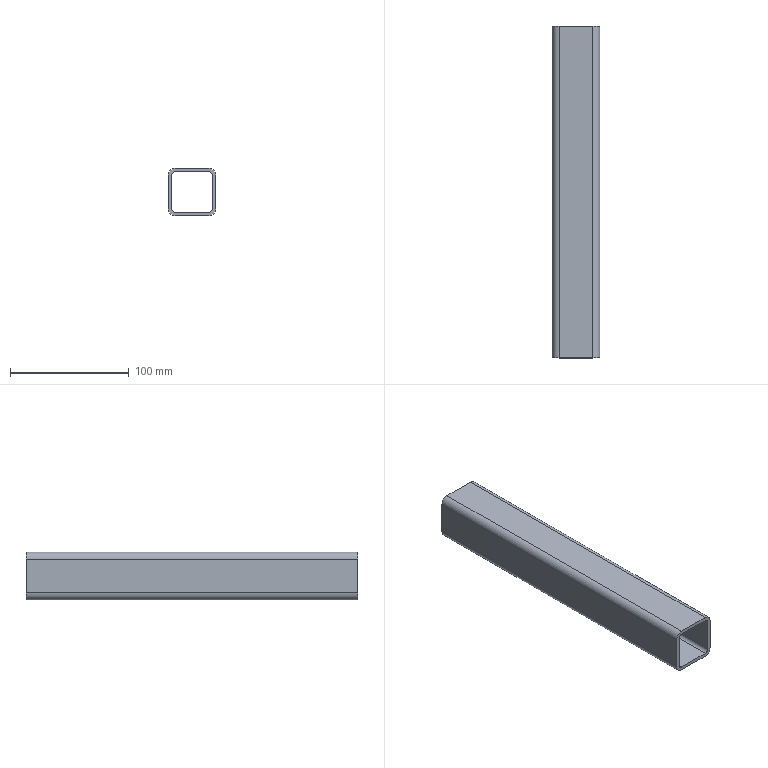Part | STEP file | SN10_002_008-05_TUBO_QUADRADO | 1 solid | 18 faces | box 40 x 280 x 40 mm | volume 117830 mm3 | plane 10 | cylinder 8 | commonest cylinder face diameters 6 x4 12 x4
STEP:
#1=CARTESIAN_POINT('',(0.,0.,0.));
#2=DIRECTION('',(0.,0.,1.));
#3=DIRECTION('',(1.,0.,0.));
#4=AXIS2_PLACEMENT_3D('',#1,#2,#3);
#5=CARTESIAN_POINT('',(14.,-140.,20.));
#6=VERTEX_POINT('',#5);
#7=CARTESIAN_POINT('',(14.,140.,20.));
#8=VERTEX_POINT('',#7);
#9=CARTESIAN_POINT('',(14.,-140.,20.));
#10=DIRECTION('',(0.,1.,0.));
#11=VECTOR('',#10,1.);
#12=LINE('',#9,#11);
#13=CARTESIAN_POINT('',(14.,0.,14.));
#14=DIRECTION('',(0.,1.,0.));
#15=DIRECTION('',(0.,0.,1.));
#16=AXIS2_PLACEMENT_3D('',#13,#14,#15);
#17=CYLINDRICAL_SURFACE('',#16,6.);
#18=CARTESIAN_POINT('',(0.,-140.));
#19=DIRECTION('',(0.,1.));
#20=VECTOR('',#19,1.);
#21=LINE('',#18,#20);
#22=(GEOMETRIC_REPRESENTATION_CONTEXT(2)PARAMETRIC_REPRESENTATION_CONTEXT()REPRESENTATION_CONTEXT('',''));
#23=DEFINITIONAL_REPRESENTATION('',(#21),#22);
#24=PCURVE('',#17,#23);
#25=CARTESIAN_POINT('',(14.,0.,20.));
#26=DIRECTION('',(0.,0.,-1.));
#27=DIRECTION('',(-1.,0.,0.));
#28=AXIS2_PLACEMENT_3D('',#25,#26,#27);
#29=PLANE('',#28);
#30=CARTESIAN_POINT('',(0.,-140.));
#31=DIRECTION('',(0.,1.));
#32=VECTOR('',#31,1.);
#33=LINE('',#30,#32);
#34=(GEOMETRIC_REPRESENTATION_CONTEXT(2)PARAMETRIC_REPRESENTATION_CONTEXT()REPRESENTATION_CONTEXT('',''));
#35=DEFINITIONAL_REPRESENTATION('',(#33),#34);
#36=PCURVE('',#29,#35);
#37=SURFACE_CURVE('',#12,(#24,#36),.PCURVE_S1.);
#38=EDGE_CURVE('',#6,#8,#37,.T.);
#39=ORIENTED_EDGE('',*,*,#38,.F.);
#40=CARTESIAN_POINT('',(20.,-140.,14.));
#41=VERTEX_POINT('',#40);
#42=CARTESIAN_POINT('',(14.,-140.,14.));
#43=DIRECTION('',(0.,1.,0.));
#44=DIRECTION('',(1.,0.,0.));
#45=AXIS2_PLACEMENT_3D('',#42,#43,#44);
#46=CIRCLE('',#45,6.);
#47=CARTESIAN_POINT('',(-4.712,-140.));
#48=DIRECTION('',(1.,0.));
#49=VECTOR('',#48,1.);
#50=LINE('',#47,#49);
#51=(GEOMETRIC_REPRESENTATION_CONTEXT(2)PARAMETRIC_REPRESENTATION_CONTEXT()REPRESENTATION_CONTEXT('',''));
#52=DEFINITIONAL_REPRESENTATION('',(#50),#51);
#53=PCURVE('',#17,#52);
#54=CARTESIAN_POINT('',(0.,-140.,0.));
#55=DIRECTION('',(0.,1.,0.));
#56=DIRECTION('',(0.,0.,1.));
#57=AXIS2_PLACEMENT_3D('',#54,#55,#56);
#58=PLANE('',#57);
#59=CARTESIAN_POINT('',(14.,14.));
#60=DIRECTION('',(0.,1.));
#61=AXIS2_PLACEMENT_2D('',#59,#60);
#62=CIRCLE('',#61,6.);
#63=(GEOMETRIC_REPRESENTATION_CONTEXT(2)PARAMETRIC_REPRESENTATION_CONTEXT()REPRESENTATION_CONTEXT('',''));
#64=DEFINITIONAL_REPRESENTATION('',(#62),#63);
#65=PCURVE('',#58,#64);
#66=SURFACE_CURVE('',#46,(#53,#65),.PCURVE_S1.);
#67=EDGE_CURVE('',#6,#41,#66,.T.);
#68=ORIENTED_EDGE('',*,*,#67,.T.);
#69=CARTESIAN_POINT('',(20.,140.,14.));
#70=VERTEX_POINT('',#69);
#71=CARTESIAN_POINT('',(20.,-140.,14.));
#72=DIRECTION('',(0.,1.,0.));
#73=VECTOR('',#72,1.);
#74=LINE('',#71,#73);
#75=CARTESIAN_POINT('',(1.571,-140.));
#76=DIRECTION('',(0.,1.));
#77=VECTOR('',#76,1.);
#78=LINE('',#75,#77);
#79=(GEOMETRIC_REPRESENTATION_CONTEXT(2)PARAMETRIC_REPRESENTATION_CONTEXT()REPRESENTATION_CONTEXT('',''));
#80=DEFINITIONAL_REPRESENTATION('',(#78),#79);
#81=PCURVE('',#17,#80);
#82=CARTESIAN_POINT('',(20.,0.,-14.));
#83=DIRECTION('',(-1.,0.,0.));
#84=DIRECTION('',(0.,0.,1.));
#85=AXIS2_PLACEMENT_3D('',#82,#83,#84);
#86=PLANE('',#85);
#87=CARTESIAN_POINT('',(28.,-140.));
#88=DIRECTION('',(0.,1.));
#89=VECTOR('',#88,1.);
#90=LINE('',#87,#89);
#91=(GEOMETRIC_REPRESENTATION_CONTEXT(2)PARAMETRIC_REPRESENTATION_CONTEXT()REPRESENTATION_CONTEXT('',''));
#92=DEFINITIONAL_REPRESENTATION('',(#90),#91);
#93=PCURVE('',#86,#92);
#94=SURFACE_CURVE('',#74,(#81,#93),.PCURVE_S1.);
#95=EDGE_CURVE('',#41,#70,#94,.T.);
#96=ORIENTED_EDGE('',*,*,#95,.T.);
#97=CARTESIAN_POINT('',(14.,140.,14.));
#98=DIRECTION('',(0.,1.,0.));
#99=DIRECTION('',(1.,0.,0.));
#100=AXIS2_PLACEMENT_3D('',#97,#98,#99);
#101=CIRCLE('',#100,6.);
#102=CARTESIAN_POINT('',(-4.712,140.));
#103=DIRECTION('',(1.,0.));
#104=VECTOR('',#103,1.);
#105=LINE('',#102,#104);
#106=(GEOMETRIC_REPRESENTATION_CONTEXT(2)PARAMETRIC_REPRESENTATION_CONTEXT()REPRESENTATION_CONTEXT('',''));
#107=DEFINITIONAL_REPRESENTATION('',(#105),#106);
#108=PCURVE('',#17,#107);
#109=CARTESIAN_POINT('',(0.,140.,0.));
#110=DIRECTION('',(0.,1.,0.));
#111=DIRECTION('',(0.,0.,1.));
#112=AXIS2_PLACEMENT_3D('',#109,#110,#111);
#113=PLANE('',#112);
#114=CARTESIAN_POINT('',(14.,14.));
#115=DIRECTION('',(0.,1.));
#116=AXIS2_PLACEMENT_2D('',#114,#115);
#117=CIRCLE('',#116,6.);
#118=(GEOMETRIC_REPRESENTATION_CONTEXT(2)PARAMETRIC_REPRESENTATION_CONTEXT()REPRESENTATION_CONTEXT('',''));
#119=DEFINITIONAL_REPRESENTATION('',(#117),#118);
#120=PCURVE('',#113,#119);
#121=SURFACE_CURVE('',#101,(#108,#120),.PCURVE_S1.);
#122=EDGE_CURVE('',#8,#70,#121,.T.);
#123=ORIENTED_EDGE('',*,*,#122,.F.);
#124=EDGE_LOOP('',(#39,#68,#96,#123));
#125=FACE_BOUND('',#124,.T.);
#126=ADVANCED_FACE('',(#125),#17,.T.);
#127=ORIENTED_EDGE('',*,*,#95,.F.);
#128=CARTESIAN_POINT('',(20.,-140.,-14.));
#129=VERTEX_POINT('',#128);
#130=CARTESIAN_POINT('',(20.,-140.,-14.));
#131=DIRECTION('',(0.,0.,1.));
#132=VECTOR('',#131,1.);
#133=LINE('',#130,#132);
#134=CARTESIAN_POINT('',(0.,-140.));
#135=DIRECTION('',(1.,0.));
#136=VECTOR('',#135,1.);
#137=LINE('',#134,#136);
#138=(GEOMETRIC_REPRESENTATION_CONTEXT(2)PARAMETRIC_REPRESENTATION_CONTEXT()REPRESENTATION_CONTEXT('',''));
#139=DEFINITIONAL_REPRESENTATION('',(#137),#138);
#140=PCURVE('',#86,#139);
#141=CARTESIAN_POINT('',(-14.,20.));
#142=DIRECTION('',(1.,0.));
#143=VECTOR('',#142,1.);
#144=LINE('',#141,#143);
#145=(GEOMETRIC_REPRESENTATION_CONTEXT(2)PARAMETRIC_REPRESENTATION_CONTEXT()REPRESENTATION_CONTEXT('',''));
#146=DEFINITIONAL_REPRESENTATION('',(#144),#145);
#147=PCURVE('',#58,#146);
#148=SURFACE_CURVE('',#133,(#140,#147),.PCURVE_S1.);
#149=EDGE_CURVE('',#129,#41,#148,.T.);
#150=ORIENTED_EDGE('',*,*,#149,.F.);
#151=CARTESIAN_POINT('',(20.,140.,-14.));
#152=VERTEX_POINT('',#151);
#153=CARTESIAN_POINT('',(20.,-140.,-14.));
#154=DIRECTION('',(0.,1.,0.));
#155=VECTOR('',#154,1.);
#156=LINE('',#153,#155);
#157=CARTESIAN_POINT('',(0.,-140.));
#158=DIRECTION('',(0.,1.));
#159=VECTOR('',#158,1.);
#160=LINE('',#157,#159);
#161=(GEOMETRIC_REPRESENTATION_CONTEXT(2)PARAMETRIC_REPRESENTATION_CONTEXT()REPRESENTATION_CONTEXT('',''));
#162=DEFINITIONAL_REPRESENTATION('',(#160),#161);
#163=PCURVE('',#86,#162);
#164=CARTESIAN_POINT('',(14.,0.,-14.));
#165=DIRECTION('',(0.,1.,0.));
#166=DIRECTION('',(1.,0.,0.));
#167=AXIS2_PLACEMENT_3D('',#164,#165,#166);
#168=CYLINDRICAL_SURFACE('',#167,6.);
#169=CARTESIAN_POINT('',(0.,-140.));
#170=DIRECTION('',(0.,1.));
#171=VECTOR('',#170,1.);
#172=LINE('',#169,#171);
#173=(GEOMETRIC_REPRESENTATION_CONTEXT(2)PARAMETRIC_REPRESENTATION_CONTEXT()REPRESENTATION_CONTEXT('',''));
#174=DEFINITIONAL_REPRESENTATION('',(#172),#173);
#175=PCURVE('',#168,#174);
#176=SURFACE_CURVE('',#156,(#163,#175),.PCURVE_S1.);
#177=EDGE_CURVE('',#129,#152,#176,.T.);
#178=ORIENTED_EDGE('',*,*,#177,.T.);
#179=CARTESIAN_POINT('',(20.,140.,-14.));
#180=DIRECTION('',(0.,0.,1.));
#181=VECTOR('',#180,1.);
#182=LINE('',#179,#181);
#183=CARTESIAN_POINT('',(0.,140.));
#184=DIRECTION('',(1.,0.));
#185=VECTOR('',#184,1.);
#186=LINE('',#183,#185);
#187=(GEOMETRIC_REPRESENTATION_CONTEXT(2)PARAMETRIC_REPRESENTATION_CONTEXT()REPRESENTATION_CONTEXT('',''));
#188=DEFINITIONAL_REPRESENTATION('',(#186),#187);
#189=PCURVE('',#86,#188);
#190=CARTESIAN_POINT('',(-14.,20.));
#191=DIRECTION('',(1.,0.));
#192=VECTOR('',#191,1.);
#193=LINE('',#190,#192);
#194=(GEOMETRIC_REPRESENTATION_CONTEXT(2)PARAMETRIC_REPRESENTATION_CONTEXT()REPRESENTATION_CONTEXT('',''));
#195=DEFINITIONAL_REPRESENTATION('',(#193),#194);
#196=PCURVE('',#113,#195);
#197=SURFACE_CURVE('',#182,(#189,#196),.PCURVE_S1.);
#198=EDGE_CURVE('',#152,#70,#197,.T.);
#199=ORIENTED_EDGE('',*,*,#198,.T.);
#200=EDGE_LOOP('',(#127,#150,#178,#199));
#201=FACE_BOUND('',#200,.T.);
#202=ADVANCED_FACE('',(#201),#86,.F.);
#203=ORIENTED_EDGE('',*,*,#177,.F.);
#204=CARTESIAN_POINT('',(14.,-140.,-20.));
#205=VERTEX_POINT('',#204);
#206=CARTESIAN_POINT('',(14.,-140.,-14.));
#207=DIRECTION('',(0.,1.,0.));
#208=DIRECTION('',(1.,0.,0.));
#209=AXIS2_PLACEMENT_3D('',#206,#207,#208);
#210=CIRCLE('',#209,6.);
#211=CARTESIAN_POINT('',(0.,-140.));
#212=DIRECTION('',(1.,0.));
#213=VECTOR('',#212,1.);
#214=LINE('',#211,#213);
#215=(GEOMETRIC_REPRESENTATION_CONTEXT(2)PARAMETRIC_REPRESENTATION_CONTEXT()REPRESENTATION_CONTEXT('',''));
#216=DEFINITIONAL_REPRESENTATION('',(#214),#215);
#217=PCURVE('',#168,#216);
#218=CARTESIAN_POINT('',(-14.,14.));
#219=DIRECTION('',(0.,1.));
#220=AXIS2_PLACEMENT_2D('',#218,#219);
#221=CIRCLE('',#220,6.);
#222=(GEOMETRIC_REPRESENTATION_CONTEXT(2)PARAMETRIC_REPRESENTATION_CONTEXT()REPRESENTATION_CONTEXT('',''));
#223=DEFINITIONAL_REPRESENTATION('',(#221),#222);
#224=PCURVE('',#58,#223);
#225=SURFACE_CURVE('',#210,(#217,#224),.PCURVE_S1.);
#226=EDGE_CURVE('',#129,#205,#225,.T.);
#227=ORIENTED_EDGE('',*,*,#226,.T.);
#228=CARTESIAN_POINT('',(14.,140.,-20.));
#229=VERTEX_POINT('',#228);
#230=CARTESIAN_POINT('',(14.,-140.,-20.));
#231=DIRECTION('',(0.,1.,0.));
#232=VECTOR('',#231,1.);
#233=LINE('',#230,#232);
#234=CARTESIAN_POINT('',(1.571,-140.));
#235=DIRECTION('',(0.,1.));
#236=VECTOR('',#235,1.);
#237=LINE('',#234,#236);
#238=(GEOMETRIC_REPRESENTATION_CONTEXT(2)PARAMETRIC_REPRESENTATION_CONTEXT()REPRESENTATION_CONTEXT('',''));
#239=DEFINITIONAL_REPRESENTATION('',(#237),#238);
#240=PCURVE('',#168,#239);
#241=CARTESIAN_POINT('',(-14.,0.,-20.));
#242=DIRECTION('',(0.,0.,1.));
#243=DIRECTION('',(1.,0.,0.));
#244=AXIS2_PLACEMENT_3D('',#241,#242,#243);
#245=PLANE('',#244);
#246=CARTESIAN_POINT('',(28.,-140.));
#247=DIRECTION('',(0.,1.));
#248=VECTOR('',#247,1.);
#249=LINE('',#246,#248);
#250=(GEOMETRIC_REPRESENTATION_CONTEXT(2)PARAMETRIC_REPRESENTATION_CONTEXT()REPRESENTATION_CONTEXT('',''));
#251=DEFINITIONAL_REPRESENTATION('',(#249),#250);
#252=PCURVE('',#245,#251);
#253=SURFACE_CURVE('',#233,(#240,#252),.PCURVE_S1.);
#254=EDGE_CURVE('',#205,#229,#253,.T.);
#255=ORIENTED_EDGE('',*,*,#254,.T.);
#256=CARTESIAN_POINT('',(14.,140.,-14.));
#257=DIRECTION('',(0.,1.,0.));
#258=DIRECTION('',(1.,0.,0.));
#259=AXIS2_PLACEMENT_3D('',#256,#257,#258);
#260=CIRCLE('',#259,6.);
#261=CARTESIAN_POINT('',(0.,140.));
#262=DIRECTION('',(1.,0.));
#263=VECTOR('',#262,1.);
#264=LINE('',#261,#263);
#265=(GEOMETRIC_REPRESENTATION_CONTEXT(2)PARAMETRIC_REPRESENTATION_CONTEXT()REPRESENTATION_CONTEXT('',''));
#266=DEFINITIONAL_REPRESENTATION('',(#264),#265);
#267=PCURVE('',#168,#266);
#268=CARTESIAN_POINT('',(-14.,14.));
#269=DIRECTION('',(0.,1.));
#270=AXIS2_PLACEMENT_2D('',#268,#269);
#271=CIRCLE('',#270,6.);
#272=(GEOMETRIC_REPRESENTATION_CONTEXT(2)PARAMETRIC_REPRESENTATION_CONTEXT()REPRESENTATION_CONTEXT('',''));
#273=DEFINITIONAL_REPRESENTATION('',(#271),#272);
#274=PCURVE('',#113,#273);
#275=SURFACE_CURVE('',#260,(#267,#274),.PCURVE_S1.);
#276=EDGE_CURVE('',#152,#229,#275,.T.);
#277=ORIENTED_EDGE('',*,*,#276,.F.);
#278=EDGE_LOOP('',(#203,#227,#255,#277));
#279=FACE_BOUND('',#278,.T.);
#280=ADVANCED_FACE('',(#279),#168,.T.);
#281=ORIENTED_EDGE('',*,*,#254,.F.);
#282=CARTESIAN_POINT('',(-14.,-140.,-20.));
#283=VERTEX_POINT('',#282);
#284=CARTESIAN_POINT('',(-14.,-140.,-20.));
#285=DIRECTION('',(1.,0.,0.));
#286=VECTOR('',#285,1.);
#287=LINE('',#284,#286);
#288=CARTESIAN_POINT('',(0.,-140.));
#289=DIRECTION('',(1.,0.));
#290=VECTOR('',#289,1.);
#291=LINE('',#288,#290);
#292=(GEOMETRIC_REPRESENTATION_CONTEXT(2)PARAMETRIC_REPRESENTATION_CONTEXT()REPRESENTATION_CONTEXT('',''));
#293=DEFINITIONAL_REPRESENTATION('',(#291),#292);
#294=PCURVE('',#245,#293);
#295=CARTESIAN_POINT('',(-20.,-14.));
#296=DIRECTION('',(0.,1.));
#297=VECTOR('',#296,1.);
#298=LINE('',#295,#297);
#299=(GEOMETRIC_REPRESENTATION_CONTEXT(2)PARAMETRIC_REPRESENTATION_CONTEXT()REPRESENTATION_CONTEXT('',''));
#300=DEFINITIONAL_REPRESENTATION('',(#298),#299);
#301=PCURVE('',#58,#300);
#302=SURFACE_CURVE('',#287,(#294,#301),.PCURVE_S1.);
#303=EDGE_CURVE('',#283,#205,#302,.T.);
#304=ORIENTED_EDGE('',*,*,#303,.F.);
#305=CARTESIAN_POINT('',(-14.,140.,-20.));
#306=VERTEX_POINT('',#305);
#307=CARTESIAN_POINT('',(-14.,-140.,-20.));
#308=DIRECTION('',(0.,1.,0.));
#309=VECTOR('',#308,1.);
#310=LINE('',#307,#309);
#311=CARTESIAN_POINT('',(0.,-140.));
#312=DIRECTION('',(0.,1.));
#313=VECTOR('',#312,1.);
#314=LINE('',#311,#313);
#315=(GEOMETRIC_REPRESENTATION_CONTEXT(2)PARAMETRIC_REPRESENTATION_CONTEXT()REPRESENTATION_CONTEXT('',''));
#316=DEFINITIONAL_REPRESENTATION('',(#314),#315);
#317=PCURVE('',#245,#316);
#318=CARTESIAN_POINT('',(-14.,0.,-14.));
#319=DIRECTION('',(0.,1.,0.));
#320=DIRECTION('',(0.,0.,-1.));
#321=AXIS2_PLACEMENT_3D('',#318,#319,#320);
#322=CYLINDRICAL_SURFACE('',#321,6.);
#323=CARTESIAN_POINT('',(0.,-140.));
#324=DIRECTION('',(0.,1.));
#325=VECTOR('',#324,1.);
#326=LINE('',#323,#325);
#327=(GEOMETRIC_REPRESENTATION_CONTEXT(2)PARAMETRIC_REPRESENTATION_CONTEXT()REPRESENTATION_CONTEXT('',''));
#328=DEFINITIONAL_REPRESENTATION('',(#326),#327);
#329=PCURVE('',#322,#328);
#330=SURFACE_CURVE('',#310,(#317,#329),.PCURVE_S1.);
#331=EDGE_CURVE('',#283,#306,#330,.T.);
#332=ORIENTED_EDGE('',*,*,#331,.T.);
#333=CARTESIAN_POINT('',(-14.,140.,-20.));
#334=DIRECTION('',(1.,0.,0.));
#335=VECTOR('',#334,1.);
#336=LINE('',#333,#335);
#337=CARTESIAN_POINT('',(0.,140.));
#338=DIRECTION('',(1.,0.));
#339=VECTOR('',#338,1.);
#340=LINE('',#337,#339);
#341=(GEOMETRIC_REPRESENTATION_CONTEXT(2)PARAMETRIC_REPRESENTATION_CONTEXT()REPRESENTATION_CONTEXT('',''));
#342=DEFINITIONAL_REPRESENTATION('',(#340),#341);
#343=PCURVE('',#245,#342);
#344=CARTESIAN_POINT('',(-20.,-14.));
#345=DIRECTION('',(0.,1.));
#346=VECTOR('',#345,1.);
#347=LINE('',#344,#346);
#348=(GEOMETRIC_REPRESENTATION_CONTEXT(2)PARAMETRIC_REPRESENTATION_CONTEXT()REPRESENTATION_CONTEXT('',''));
#349=DEFINITIONAL_REPRESENTATION('',(#347),#348);
#350=PCURVE('',#113,#349);
#351=SURFACE_CURVE('',#336,(#343,#350),.PCURVE_S1.);
#352=EDGE_CURVE('',#306,#229,#351,.T.);
#353=ORIENTED_EDGE('',*,*,#352,.T.);
#354=EDGE_LOOP('',(#281,#304,#332,#353));
#355=FACE_BOUND('',#354,.T.);
#356=ADVANCED_FACE('',(#355),#245,.F.);
#357=ORIENTED_EDGE('',*,*,#331,.F.);
#358=CARTESIAN_POINT('',(-20.,-140.,-14.));
#359=VERTEX_POINT('',#358);
#360=CARTESIAN_POINT('',(-14.,-140.,-14.));
#361=DIRECTION('',(0.,1.,0.));
#362=DIRECTION('',(1.,0.,0.));
#363=AXIS2_PLACEMENT_3D('',#360,#361,#362);
#364=CIRCLE('',#363,6.);
#365=CARTESIAN_POINT('',(-1.571,-140.));
#366=DIRECTION('',(1.,0.));
#367=VECTOR('',#366,1.);
#368=LINE('',#365,#367);
#369=(GEOMETRIC_REPRESENTATION_CONTEXT(2)PARAMETRIC_REPRESENTATION_CONTEXT()REPRESENTATION_CONTEXT('',''));
#370=DEFINITIONAL_REPRESENTATION('',(#368),#369);
#371=PCURVE('',#322,#370);
#372=CARTESIAN_POINT('',(-14.,-14.));
#373=DIRECTION('',(0.,1.));
#374=AXIS2_PLACEMENT_2D('',#372,#373);
#375=CIRCLE('',#374,6.);
#376=(GEOMETRIC_REPRESENTATION_CONTEXT(2)PARAMETRIC_REPRESENTATION_CONTEXT()REPRESENTATION_CONTEXT('',''));
#377=DEFINITIONAL_REPRESENTATION('',(#375),#376);
#378=PCURVE('',#58,#377);
#379=SURFACE_CURVE('',#364,(#371,#378),.PCURVE_S1.);
#380=EDGE_CURVE('',#283,#359,#379,.T.);
#381=ORIENTED_EDGE('',*,*,#380,.T.);
#382=CARTESIAN_POINT('',(-20.,140.,-14.));
#383=VERTEX_POINT('',#382);
#384=CARTESIAN_POINT('',(-20.,-140.,-14.));
#385=DIRECTION('',(0.,1.,0.));
#386=VECTOR('',#385,1.);
#387=LINE('',#384,#386);
#388=CARTESIAN_POINT('',(1.571,-140.));
#389=DIRECTION('',(0.,1.));
#390=VECTOR('',#389,1.);
#391=LINE('',#388,#390);
#392=(GEOMETRIC_REPRESENTATION_CONTEXT(2)PARAMETRIC_REPRESENTATION_CONTEXT()REPRESENTATION_CONTEXT('',''));
#393=DEFINITIONAL_REPRESENTATION('',(#391),#392);
#394=PCURVE('',#322,#393);
#395=CARTESIAN_POINT('',(-20.,0.,14.));
#396=DIRECTION('',(1.,0.,0.));
#397=DIRECTION('',(0.,0.,-1.));
#398=AXIS2_PLACEMENT_3D('',#395,#396,#397);
#399=PLANE('',#398);
#400=CARTESIAN_POINT('',(28.,-140.));
#401=DIRECTION('',(0.,1.));
#402=VECTOR('',#401,1.);
#403=LINE('',#400,#402);
#404=(GEOMETRIC_REPRESENTATION_CONTEXT(2)PARAMETRIC_REPRESENTATION_CONTEXT()REPRESENTATION_CONTEXT('',''));
#405=DEFINITIONAL_REPRESENTATION('',(#403),#404);
#406=PCURVE('',#399,#405);
#407=SURFACE_CURVE('',#387,(#394,#406),.PCURVE_S1.);
#408=EDGE_CURVE('',#359,#383,#407,.T.);
#409=ORIENTED_EDGE('',*,*,#408,.T.);
#410=CARTESIAN_POINT('',(-14.,140.,-14.));
#411=DIRECTION('',(0.,1.,0.));
#412=DIRECTION('',(1.,0.,0.));
#413=AXIS2_PLACEMENT_3D('',#410,#411,#412);
#414=CIRCLE('',#413,6.);
#415=CARTESIAN_POINT('',(-1.571,140.));
#416=DIRECTION('',(1.,0.));
#417=VECTOR('',#416,1.);
#418=LINE('',#415,#417);
#419=(GEOMETRIC_REPRESENTATION_CONTEXT(2)PARAMETRIC_REPRESENTATION_CONTEXT()REPRESENTATION_CONTEXT('',''));
#420=DEFINITIONAL_REPRESENTATION('',(#418),#419);
#421=PCURVE('',#322,#420);
#422=CARTESIAN_POINT('',(-14.,-14.));
#423=DIRECTION('',(0.,1.));
#424=AXIS2_PLACEMENT_2D('',#422,#423);
#425=CIRCLE('',#424,6.);
#426=(GEOMETRIC_REPRESENTATION_CONTEXT(2)PARAMETRIC_REPRESENTATION_CONTEXT()REPRESENTATION_CONTEXT('',''));
#427=DEFINITIONAL_REPRESENTATION('',(#425),#426);
#428=PCURVE('',#113,#427);
#429=SURFACE_CURVE('',#414,(#421,#428),.PCURVE_S1.);
#430=EDGE_CURVE('',#306,#383,#429,.T.);
#431=ORIENTED_EDGE('',*,*,#430,.F.);
#432=EDGE_LOOP('',(#357,#381,#409,#431));
#433=FACE_BOUND('',#432,.T.);
#434=ADVANCED_FACE('',(#433),#322,.T.);
#435=ORIENTED_EDGE('',*,*,#408,.F.);
#436=CARTESIAN_POINT('',(-20.,-140.,14.));
#437=VERTEX_POINT('',#436);
#438=CARTESIAN_POINT('',(-20.,-140.,14.));
#439=DIRECTION('',(0.,0.,-1.));
#440=VECTOR('',#439,1.);
#441=LINE('',#438,#440);
#442=CARTESIAN_POINT('',(0.,-140.));
#443=DIRECTION('',(1.,0.));
#444=VECTOR('',#443,1.);
#445=LINE('',#442,#444);
#446=(GEOMETRIC_REPRESENTATION_CONTEXT(2)PARAMETRIC_REPRESENTATION_CONTEXT()REPRESENTATION_CONTEXT('',''));
#447=DEFINITIONAL_REPRESENTATION('',(#445),#446);
#448=PCURVE('',#399,#447);
#449=CARTESIAN_POINT('',(14.,-20.));
#450=DIRECTION('',(-1.,0.));
#451=VECTOR('',#450,1.);
#452=LINE('',#449,#451);
#453=(GEOMETRIC_REPRESENTATION_CONTEXT(2)PARAMETRIC_REPRESENTATION_CONTEXT()REPRESENTATION_CONTEXT('',''));
#454=DEFINITIONAL_REPRESENTATION('',(#452),#453);
#455=PCURVE('',#58,#454);
#456=SURFACE_CURVE('',#441,(#448,#455),.PCURVE_S1.);
#457=EDGE_CURVE('',#437,#359,#456,.T.);
#458=ORIENTED_EDGE('',*,*,#457,.F.);
#459=CARTESIAN_POINT('',(-20.,140.,14.));
#460=VERTEX_POINT('',#459);
#461=CARTESIAN_POINT('',(-20.,-140.,14.));
#462=DIRECTION('',(0.,1.,0.));
#463=VECTOR('',#462,1.);
#464=LINE('',#461,#463);
#465=CARTESIAN_POINT('',(0.,-140.));
#466=DIRECTION('',(0.,1.));
#467=VECTOR('',#466,1.);
#468=LINE('',#465,#467);
#469=(GEOMETRIC_REPRESENTATION_CONTEXT(2)PARAMETRIC_REPRESENTATION_CONTEXT()REPRESENTATION_CONTEXT('',''));
#470=DEFINITIONAL_REPRESENTATION('',(#468),#469);
#471=PCURVE('',#399,#470);
#472=CARTESIAN_POINT('',(-14.,0.,14.));
#473=DIRECTION('',(0.,1.,0.));
#474=DIRECTION('',(-1.,0.,0.));
#475=AXIS2_PLACEMENT_3D('',#472,#473,#474);
#476=CYLINDRICAL_SURFACE('',#475,6.);
#477=CARTESIAN_POINT('',(0.,-140.));
#478=DIRECTION('',(0.,1.));
#479=VECTOR('',#478,1.);
#480=LINE('',#477,#479);
#481=(GEOMETRIC_REPRESENTATION_CONTEXT(2)PARAMETRIC_REPRESENTATION_CONTEXT()REPRESENTATION_CONTEXT('',''));
#482=DEFINITIONAL_REPRESENTATION('',(#480),#481);
#483=PCURVE('',#476,#482);
#484=SURFACE_CURVE('',#464,(#471,#483),.PCURVE_S1.);
#485=EDGE_CURVE('',#437,#460,#484,.T.);
#486=ORIENTED_EDGE('',*,*,#485,.T.);
#487=CARTESIAN_POINT('',(-20.,140.,14.));
#488=DIRECTION('',(0.,0.,-1.));
#489=VECTOR('',#488,1.);
#490=LINE('',#487,#489);
#491=CARTESIAN_POINT('',(0.,140.));
#492=DIRECTION('',(1.,0.));
#493=VECTOR('',#492,1.);
#494=LINE('',#491,#493);
#495=(GEOMETRIC_REPRESENTATION_CONTEXT(2)PARAMETRIC_REPRESENTATION_CONTEXT()REPRESENTATION_CONTEXT('',''));
#496=DEFINITIONAL_REPRESENTATION('',(#494),#495);
#497=PCURVE('',#399,#496);
#498=CARTESIAN_POINT('',(14.,-20.));
#499=DIRECTION('',(-1.,0.));
#500=VECTOR('',#499,1.);
#501=LINE('',#498,#500);
#502=(GEOMETRIC_REPRESENTATION_CONTEXT(2)PARAMETRIC_REPRESENTATION_CONTEXT()REPRESENTATION_CONTEXT('',''));
#503=DEFINITIONAL_REPRESENTATION('',(#501),#502);
#504=PCURVE('',#113,#503);
#505=SURFACE_CURVE('',#490,(#497,#504),.PCURVE_S1.);
#506=EDGE_CURVE('',#460,#383,#505,.T.);
#507=ORIENTED_EDGE('',*,*,#506,.T.);
#508=EDGE_LOOP('',(#435,#458,#486,#507));
#509=FACE_BOUND('',#508,.T.);
#510=ADVANCED_FACE('',(#509),#399,.F.);
#511=ORIENTED_EDGE('',*,*,#485,.F.);
#512=CARTESIAN_POINT('',(-14.,-140.,20.));
#513=VERTEX_POINT('',#512);
#514=CARTESIAN_POINT('',(-14.,-140.,14.));
#515=DIRECTION('',(0.,1.,0.));
#516=DIRECTION('',(1.,0.,0.));
#517=AXIS2_PLACEMENT_3D('',#514,#515,#516);
#518=CIRCLE('',#517,6.);
#519=CARTESIAN_POINT('',(-3.142,-140.));
#520=DIRECTION('',(1.,0.));
#521=VECTOR('',#520,1.);
#522=LINE('',#519,#521);
#523=(GEOMETRIC_REPRESENTATION_CONTEXT(2)PARAMETRIC_REPRESENTATION_CONTEXT()REPRESENTATION_CONTEXT('',''));
#524=DEFINITIONAL_REPRESENTATION('',(#522),#523);
#525=PCURVE('',#476,#524);
#526=CARTESIAN_POINT('',(14.,-14.));
#527=DIRECTION('',(0.,1.));
#528=AXIS2_PLACEMENT_2D('',#526,#527);
#529=CIRCLE('',#528,6.);
#530=(GEOMETRIC_REPRESENTATION_CONTEXT(2)PARAMETRIC_REPRESENTATION_CONTEXT()REPRESENTATION_CONTEXT('',''));
#531=DEFINITIONAL_REPRESENTATION('',(#529),#530);
#532=PCURVE('',#58,#531);
#533=SURFACE_CURVE('',#518,(#525,#532),.PCURVE_S1.);
#534=EDGE_CURVE('',#437,#513,#533,.T.);
#535=ORIENTED_EDGE('',*,*,#534,.T.);
#536=CARTESIAN_POINT('',(-14.,140.,20.));
#537=VERTEX_POINT('',#536);
#538=CARTESIAN_POINT('',(-14.,-140.,20.));
#539=DIRECTION('',(0.,1.,0.));
#540=VECTOR('',#539,1.);
#541=LINE('',#538,#540);
#542=CARTESIAN_POINT('',(1.571,-140.));
#543=DIRECTION('',(0.,1.));
#544=VECTOR('',#543,1.);
#545=LINE('',#542,#544);
#546=(GEOMETRIC_REPRESENTATION_CONTEXT(2)PARAMETRIC_REPRESENTATION_CONTEXT()REPRESENTATION_CONTEXT('',''));
#547=DEFINITIONAL_REPRESENTATION('',(#545),#546);
#548=PCURVE('',#476,#547);
#549=CARTESIAN_POINT('',(28.,-140.));
#550=DIRECTION('',(0.,1.));
#551=VECTOR('',#550,1.);
#552=LINE('',#549,#551);
#553=(GEOMETRIC_REPRESENTATION_CONTEXT(2)PARAMETRIC_REPRESENTATION_CONTEXT()REPRESENTATION_CONTEXT('',''));
#554=DEFINITIONAL_REPRESENTATION('',(#552),#553);
#555=PCURVE('',#29,#554);
#556=SURFACE_CURVE('',#541,(#548,#555),.PCURVE_S1.);
#557=EDGE_CURVE('',#513,#537,#556,.T.);
#558=ORIENTED_EDGE('',*,*,#557,.T.);
#559=CARTESIAN_POINT('',(-14.,140.,14.));
#560=DIRECTION('',(0.,1.,0.));
#561=DIRECTION('',(1.,0.,0.));
#562=AXIS2_PLACEMENT_3D('',#559,#560,#561);
#563=CIRCLE('',#562,6.);
#564=CARTESIAN_POINT('',(-3.142,140.));
#565=DIRECTION('',(1.,0.));
#566=VECTOR('',#565,1.);
#567=LINE('',#564,#566);
#568=(GEOMETRIC_REPRESENTATION_CONTEXT(2)PARAMETRIC_REPRESENTATION_CONTEXT()REPRESENTATION_CONTEXT('',''));
#569=DEFINITIONAL_REPRESENTATION('',(#567),#568);
#570=PCURVE('',#476,#569);
#571=CARTESIAN_POINT('',(14.,-14.));
#572=DIRECTION('',(0.,1.));
#573=AXIS2_PLACEMENT_2D('',#571,#572);
#574=CIRCLE('',#573,6.);
#575=(GEOMETRIC_REPRESENTATION_CONTEXT(2)PARAMETRIC_REPRESENTATION_CONTEXT()REPRESENTATION_CONTEXT('',''));
#576=DEFINITIONAL_REPRESENTATION('',(#574),#575);
#577=PCURVE('',#113,#576);
#578=SURFACE_CURVE('',#563,(#570,#577),.PCURVE_S1.);
#579=EDGE_CURVE('',#460,#537,#578,.T.);
#580=ORIENTED_EDGE('',*,*,#579,.F.);
#581=EDGE_LOOP('',(#511,#535,#558,#580));
#582=FACE_BOUND('',#581,.T.);
#583=ADVANCED_FACE('',(#582),#476,.T.);
#584=ORIENTED_EDGE('',*,*,#557,.F.);
#585=CARTESIAN_POINT('',(14.,-140.,20.));
#586=DIRECTION('',(-1.,0.,0.));
#587=VECTOR('',#586,1.);
#588=LINE('',#585,#587);
#589=CARTESIAN_POINT('',(0.,-140.));
#590=DIRECTION('',(1.,0.));
#591=VECTOR('',#590,1.);
#592=LINE('',#589,#591);
#593=(GEOMETRIC_REPRESENTATION_CONTEXT(2)PARAMETRIC_REPRESENTATION_CONTEXT()REPRESENTATION_CONTEXT('',''));
#594=DEFINITIONAL_REPRESENTATION('',(#592),#593);
#595=PCURVE('',#29,#594);
#596=CARTESIAN_POINT('',(20.,14.));
#597=DIRECTION('',(0.,-1.));
#598=VECTOR('',#597,1.);
#599=LINE('',#596,#598);
#600=(GEOMETRIC_REPRESENTATION_CONTEXT(2)PARAMETRIC_REPRESENTATION_CONTEXT()REPRESENTATION_CONTEXT('',''));
#601=DEFINITIONAL_REPRESENTATION('',(#599),#600);
#602=PCURVE('',#58,#601);
#603=SURFACE_CURVE('',#588,(#595,#602),.PCURVE_S1.);
#604=EDGE_CURVE('',#6,#513,#603,.T.);
#605=ORIENTED_EDGE('',*,*,#604,.F.);
#606=ORIENTED_EDGE('',*,*,#38,.T.);
#607=CARTESIAN_POINT('',(14.,140.,20.));
#608=DIRECTION('',(-1.,0.,0.));
#609=VECTOR('',#608,1.);
#610=LINE('',#607,#609);
#611=CARTESIAN_POINT('',(0.,140.));
#612=DIRECTION('',(1.,0.));
#613=VECTOR('',#612,1.);
#614=LINE('',#611,#613);
#615=(GEOMETRIC_REPRESENTATION_CONTEXT(2)PARAMETRIC_REPRESENTATION_CONTEXT()REPRESENTATION_CONTEXT('',''));
#616=DEFINITIONAL_REPRESENTATION('',(#614),#615);
#617=PCURVE('',#29,#616);
#618=CARTESIAN_POINT('',(20.,14.));
#619=DIRECTION('',(0.,-1.));
#620=VECTOR('',#619,1.);
#621=LINE('',#618,#620);
#622=(GEOMETRIC_REPRESENTATION_CONTEXT(2)PARAMETRIC_REPRESENTATION_CONTEXT()REPRESENTATION_CONTEXT('',''));
#623=DEFINITIONAL_REPRESENTATION('',(#621),#622);
#624=PCURVE('',#113,#623);
#625=SURFACE_CURVE('',#610,(#617,#624),.PCURVE_S1.);
#626=EDGE_CURVE('',#8,#537,#625,.T.);
#627=ORIENTED_EDGE('',*,*,#626,.T.);
#628=EDGE_LOOP('',(#584,#605,#606,#627));
#629=FACE_BOUND('',#628,.T.);
#630=ADVANCED_FACE('',(#629),#29,.F.);
#631=CARTESIAN_POINT('',(14.,140.,17.));
#632=VERTEX_POINT('',#631);
#633=CARTESIAN_POINT('',(-14.,140.,17.));
#634=VERTEX_POINT('',#633);
#635=CARTESIAN_POINT('',(14.,140.,17.));
#636=DIRECTION('',(-1.,0.,0.));
#637=VECTOR('',#636,1.);
#638=LINE('',#635,#637);
#639=CARTESIAN_POINT('',(14.,0.,17.));
#640=DIRECTION('',(0.,0.,-1.));
#641=DIRECTION('',(-1.,0.,0.));
#642=AXIS2_PLACEMENT_3D('',#639,#640,#641);
#643=PLANE('',#642);
#644=CARTESIAN_POINT('',(0.,140.));
#645=DIRECTION('',(1.,0.));
#646=VECTOR('',#645,1.);
#647=LINE('',#644,#646);
#648=(GEOMETRIC_REPRESENTATION_CONTEXT(2)PARAMETRIC_REPRESENTATION_CONTEXT()REPRESENTATION_CONTEXT('',''));
#649=DEFINITIONAL_REPRESENTATION('',(#647),#648);
#650=PCURVE('',#643,#649);
#651=CARTESIAN_POINT('',(17.,14.));
#652=DIRECTION('',(0.,-1.));
#653=VECTOR('',#652,1.);
#654=LINE('',#651,#653);
#655=(GEOMETRIC_REPRESENTATION_CONTEXT(2)PARAMETRIC_REPRESENTATION_CONTEXT()REPRESENTATION_CONTEXT('',''));
#656=DEFINITIONAL_REPRESENTATION('',(#654),#655);
#657=PCURVE('',#113,#656);
#658=SURFACE_CURVE('',#638,(#650,#657),.PCURVE_S1.);
#659=EDGE_CURVE('',#632,#634,#658,.T.);
#660=ORIENTED_EDGE('',*,*,#659,.F.);
#661=CARTESIAN_POINT('',(14.,-140.,17.));
#662=VERTEX_POINT('',#661);
#663=CARTESIAN_POINT('',(14.,-140.,17.));
#664=DIRECTION('',(0.,1.,0.));
#665=VECTOR('',#664,1.);
#666=LINE('',#663,#665);
#667=CARTESIAN_POINT('',(0.,-140.));
#668=DIRECTION('',(0.,1.));
#669=VECTOR('',#668,1.);
#670=LINE('',#667,#669);
#671=(GEOMETRIC_REPRESENTATION_CONTEXT(2)PARAMETRIC_REPRESENTATION_CONTEXT()REPRESENTATION_CONTEXT('',''));
#672=DEFINITIONAL_REPRESENTATION('',(#670),#671);
#673=PCURVE('',#643,#672);
#674=CARTESIAN_POINT('',(14.,0.,14.));
#675=DIRECTION('',(0.,1.,0.));
#676=DIRECTION('',(0.,0.,1.));
#677=AXIS2_PLACEMENT_3D('',#674,#675,#676);
#678=CYLINDRICAL_SURFACE('',#677,3.);
#679=CARTESIAN_POINT('',(0.,-140.));
#680=DIRECTION('',(0.,1.));
#681=VECTOR('',#680,1.);
#682=LINE('',#679,#681);
#683=(GEOMETRIC_REPRESENTATION_CONTEXT(2)PARAMETRIC_REPRESENTATION_CONTEXT()REPRESENTATION_CONTEXT('',''));
#684=DEFINITIONAL_REPRESENTATION('',(#682),#683);
#685=PCURVE('',#678,#684);
#686=SURFACE_CURVE('',#666,(#673,#685),.PCURVE_S1.);
#687=EDGE_CURVE('',#662,#632,#686,.T.);
#688=ORIENTED_EDGE('',*,*,#687,.F.);
#689=CARTESIAN_POINT('',(-14.,-140.,17.));
#690=VERTEX_POINT('',#689);
#691=CARTESIAN_POINT('',(14.,-140.,17.));
#692=DIRECTION('',(-1.,0.,0.));
#693=VECTOR('',#692,1.);
#694=LINE('',#691,#693);
#695=CARTESIAN_POINT('',(0.,-140.));
#696=DIRECTION('',(1.,0.));
#697=VECTOR('',#696,1.);
#698=LINE('',#695,#697);
#699=(GEOMETRIC_REPRESENTATION_CONTEXT(2)PARAMETRIC_REPRESENTATION_CONTEXT()REPRESENTATION_CONTEXT('',''));
#700=DEFINITIONAL_REPRESENTATION('',(#698),#699);
#701=PCURVE('',#643,#700);
#702=CARTESIAN_POINT('',(17.,14.));
#703=DIRECTION('',(0.,-1.));
#704=VECTOR('',#703,1.);
#705=LINE('',#702,#704);
#706=(GEOMETRIC_REPRESENTATION_CONTEXT(2)PARAMETRIC_REPRESENTATION_CONTEXT()REPRESENTATION_CONTEXT('',''));
#707=DEFINITIONAL_REPRESENTATION('',(#705),#706);
#708=PCURVE('',#58,#707);
#709=SURFACE_CURVE('',#694,(#701,#708),.PCURVE_S1.);
#710=EDGE_CURVE('',#662,#690,#709,.T.);
#711=ORIENTED_EDGE('',*,*,#710,.T.);
#712=CARTESIAN_POINT('',(-14.,-140.,17.));
#713=DIRECTION('',(0.,1.,0.));
#714=VECTOR('',#713,1.);
#715=LINE('',#712,#714);
#716=CARTESIAN_POINT('',(28.,-140.));
#717=DIRECTION('',(0.,1.));
#718=VECTOR('',#717,1.);
#719=LINE('',#716,#718);
#720=(GEOMETRIC_REPRESENTATION_CONTEXT(2)PARAMETRIC_REPRESENTATION_CONTEXT()REPRESENTATION_CONTEXT('',''));
#721=DEFINITIONAL_REPRESENTATION('',(#719),#720);
#722=PCURVE('',#643,#721);
#723=CARTESIAN_POINT('',(-14.,0.,14.));
#724=DIRECTION('',(0.,1.,0.));
#725=DIRECTION('',(-1.,0.,0.));
#726=AXIS2_PLACEMENT_3D('',#723,#724,#725);
#727=CYLINDRICAL_SURFACE('',#726,3.);
#728=CARTESIAN_POINT('',(1.571,-140.));
#729=DIRECTION('',(0.,1.));
#730=VECTOR('',#729,1.);
#731=LINE('',#728,#730);
#732=(GEOMETRIC_REPRESENTATION_CONTEXT(2)PARAMETRIC_REPRESENTATION_CONTEXT()REPRESENTATION_CONTEXT('',''));
#733=DEFINITIONAL_REPRESENTATION('',(#731),#732);
#734=PCURVE('',#727,#733);
#735=SURFACE_CURVE('',#715,(#722,#734),.PCURVE_S1.);
#736=EDGE_CURVE('',#690,#634,#735,.T.);
#737=ORIENTED_EDGE('',*,*,#736,.T.);
#738=EDGE_LOOP('',(#660,#688,#711,#737));
#739=FACE_BOUND('',#738,.T.);
#740=ADVANCED_FACE('',(#739),#643,.T.);
#741=CARTESIAN_POINT('',(-17.,-140.,14.));
#742=VERTEX_POINT('',#741);
#743=CARTESIAN_POINT('',(-17.,140.,14.));
#744=VERTEX_POINT('',#743);
#745=CARTESIAN_POINT('',(-17.,-140.,14.));
#746=DIRECTION('',(0.,1.,0.));
#747=VECTOR('',#746,1.);
#748=LINE('',#745,#747);
#749=CARTESIAN_POINT('',(0.,-140.));
#750=DIRECTION('',(0.,1.));
#751=VECTOR('',#750,1.);
#752=LINE('',#749,#751);
#753=(GEOMETRIC_REPRESENTATION_CONTEXT(2)PARAMETRIC_REPRESENTATION_CONTEXT()REPRESENTATION_CONTEXT('',''));
#754=DEFINITIONAL_REPRESENTATION('',(#752),#753);
#755=PCURVE('',#727,#754);
#756=CARTESIAN_POINT('',(-17.,0.,14.));
#757=DIRECTION('',(1.,0.,0.));
#758=DIRECTION('',(0.,0.,-1.));
#759=AXIS2_PLACEMENT_3D('',#756,#757,#758);
#760=PLANE('',#759);
#761=CARTESIAN_POINT('',(0.,-140.));
#762=DIRECTION('',(0.,1.));
#763=VECTOR('',#762,1.);
#764=LINE('',#761,#763);
#765=(GEOMETRIC_REPRESENTATION_CONTEXT(2)PARAMETRIC_REPRESENTATION_CONTEXT()REPRESENTATION_CONTEXT('',''));
#766=DEFINITIONAL_REPRESENTATION('',(#764),#765);
#767=PCURVE('',#760,#766);
#768=SURFACE_CURVE('',#748,(#755,#767),.PCURVE_S1.);
#769=EDGE_CURVE('',#742,#744,#768,.T.);
#770=ORIENTED_EDGE('',*,*,#769,.F.);
#771=CARTESIAN_POINT('',(-14.,-140.,14.));
#772=DIRECTION('',(0.,1.,0.));
#773=DIRECTION('',(1.,0.,0.));
#774=AXIS2_PLACEMENT_3D('',#771,#772,#773);
#775=CIRCLE('',#774,3.);
#776=CARTESIAN_POINT('',(-3.142,-140.));
#777=DIRECTION('',(1.,0.));
#778=VECTOR('',#777,1.);
#779=LINE('',#776,#778);
#780=(GEOMETRIC_REPRESENTATION_CONTEXT(2)PARAMETRIC_REPRESENTATION_CONTEXT()REPRESENTATION_CONTEXT('',''));
#781=DEFINITIONAL_REPRESENTATION('',(#779),#780);
#782=PCURVE('',#727,#781);
#783=CARTESIAN_POINT('',(14.,-14.));
#784=DIRECTION('',(0.,1.));
#785=AXIS2_PLACEMENT_2D('',#783,#784);
#786=CIRCLE('',#785,3.);
#787=(GEOMETRIC_REPRESENTATION_CONTEXT(2)PARAMETRIC_REPRESENTATION_CONTEXT()REPRESENTATION_CONTEXT('',''));
#788=DEFINITIONAL_REPRESENTATION('',(#786),#787);
#789=PCURVE('',#58,#788);
#790=SURFACE_CURVE('',#775,(#782,#789),.PCURVE_S1.);
#791=EDGE_CURVE('',#742,#690,#790,.T.);
#792=ORIENTED_EDGE('',*,*,#791,.T.);
#793=ORIENTED_EDGE('',*,*,#736,.T.);
#794=CARTESIAN_POINT('',(-14.,140.,14.));
#795=DIRECTION('',(0.,1.,0.));
#796=DIRECTION('',(1.,0.,0.));
#797=AXIS2_PLACEMENT_3D('',#794,#795,#796);
#798=CIRCLE('',#797,3.);
#799=CARTESIAN_POINT('',(-3.142,140.));
#800=DIRECTION('',(1.,0.));
#801=VECTOR('',#800,1.);
#802=LINE('',#799,#801);
#803=(GEOMETRIC_REPRESENTATION_CONTEXT(2)PARAMETRIC_REPRESENTATION_CONTEXT()REPRESENTATION_CONTEXT('',''));
#804=DEFINITIONAL_REPRESENTATION('',(#802),#803);
#805=PCURVE('',#727,#804);
#806=CARTESIAN_POINT('',(14.,-14.));
#807=DIRECTION('',(0.,1.));
#808=AXIS2_PLACEMENT_2D('',#806,#807);
#809=CIRCLE('',#808,3.);
#810=(GEOMETRIC_REPRESENTATION_CONTEXT(2)PARAMETRIC_REPRESENTATION_CONTEXT()REPRESENTATION_CONTEXT('',''));
#811=DEFINITIONAL_REPRESENTATION('',(#809),#810);
#812=PCURVE('',#113,#811);
#813=SURFACE_CURVE('',#798,(#805,#812),.PCURVE_S1.);
#814=EDGE_CURVE('',#744,#634,#813,.T.);
#815=ORIENTED_EDGE('',*,*,#814,.F.);
#816=EDGE_LOOP('',(#770,#792,#793,#815));
#817=FACE_BOUND('',#816,.F.);
#818=ADVANCED_FACE('',(#817),#727,.F.);
#819=CARTESIAN_POINT('',(-17.,140.,-14.));
#820=VERTEX_POINT('',#819);
#821=CARTESIAN_POINT('',(-17.,140.,14.));
#822=DIRECTION('',(0.,0.,-1.));
#823=VECTOR('',#822,1.);
#824=LINE('',#821,#823);
#825=CARTESIAN_POINT('',(0.,140.));
#826=DIRECTION('',(1.,0.));
#827=VECTOR('',#826,1.);
#828=LINE('',#825,#827);
#829=(GEOMETRIC_REPRESENTATION_CONTEXT(2)PARAMETRIC_REPRESENTATION_CONTEXT()REPRESENTATION_CONTEXT('',''));
#830=DEFINITIONAL_REPRESENTATION('',(#828),#829);
#831=PCURVE('',#760,#830);
#832=CARTESIAN_POINT('',(14.,-17.));
#833=DIRECTION('',(-1.,0.));
#834=VECTOR('',#833,1.);
#835=LINE('',#832,#834);
#836=(GEOMETRIC_REPRESENTATION_CONTEXT(2)PARAMETRIC_REPRESENTATION_CONTEXT()REPRESENTATION_CONTEXT('',''));
#837=DEFINITIONAL_REPRESENTATION('',(#835),#836);
#838=PCURVE('',#113,#837);
#839=SURFACE_CURVE('',#824,(#831,#838),.PCURVE_S1.);
#840=EDGE_CURVE('',#744,#820,#839,.T.);
#841=ORIENTED_EDGE('',*,*,#840,.F.);
#842=ORIENTED_EDGE('',*,*,#769,.F.);
#843=CARTESIAN_POINT('',(-17.,-140.,-14.));
#844=VERTEX_POINT('',#843);
#845=CARTESIAN_POINT('',(-17.,-140.,14.));
#846=DIRECTION('',(0.,0.,-1.));
#847=VECTOR('',#846,1.);
#848=LINE('',#845,#847);
#849=CARTESIAN_POINT('',(0.,-140.));
#850=DIRECTION('',(1.,0.));
#851=VECTOR('',#850,1.);
#852=LINE('',#849,#851);
#853=(GEOMETRIC_REPRESENTATION_CONTEXT(2)PARAMETRIC_REPRESENTATION_CONTEXT()REPRESENTATION_CONTEXT('',''));
#854=DEFINITIONAL_REPRESENTATION('',(#852),#853);
#855=PCURVE('',#760,#854);
#856=CARTESIAN_POINT('',(14.,-17.));
#857=DIRECTION('',(-1.,0.));
#858=VECTOR('',#857,1.);
#859=LINE('',#856,#858);
#860=(GEOMETRIC_REPRESENTATION_CONTEXT(2)PARAMETRIC_REPRESENTATION_CONTEXT()REPRESENTATION_CONTEXT('',''));
#861=DEFINITIONAL_REPRESENTATION('',(#859),#860);
#862=PCURVE('',#58,#861);
#863=SURFACE_CURVE('',#848,(#855,#862),.PCURVE_S1.);
#864=EDGE_CURVE('',#742,#844,#863,.T.);
#865=ORIENTED_EDGE('',*,*,#864,.T.);
#866=CARTESIAN_POINT('',(-17.,-140.,-14.));
#867=DIRECTION('',(0.,1.,0.));
#868=VECTOR('',#867,1.);
#869=LINE('',#866,#868);
#870=CARTESIAN_POINT('',(28.,-140.));
#871=DIRECTION('',(0.,1.));
#872=VECTOR('',#871,1.);
#873=LINE('',#870,#872);
#874=(GEOMETRIC_REPRESENTATION_CONTEXT(2)PARAMETRIC_REPRESENTATION_CONTEXT()REPRESENTATION_CONTEXT('',''));
#875=DEFINITIONAL_REPRESENTATION('',(#873),#874);
#876=PCURVE('',#760,#875);
#877=CARTESIAN_POINT('',(-14.,0.,-14.));
#878=DIRECTION('',(0.,1.,0.));
#879=DIRECTION('',(0.,0.,-1.));
#880=AXIS2_PLACEMENT_3D('',#877,#878,#879);
#881=CYLINDRICAL_SURFACE('',#880,3.);
#882=CARTESIAN_POINT('',(1.571,-140.));
#883=DIRECTION('',(0.,1.));
#884=VECTOR('',#883,1.);
#885=LINE('',#882,#884);
#886=(GEOMETRIC_REPRESENTATION_CONTEXT(2)PARAMETRIC_REPRESENTATION_CONTEXT()REPRESENTATION_CONTEXT('',''));
#887=DEFINITIONAL_REPRESENTATION('',(#885),#886);
#888=PCURVE('',#881,#887);
#889=SURFACE_CURVE('',#869,(#876,#888),.PCURVE_S1.);
#890=EDGE_CURVE('',#844,#820,#889,.T.);
#891=ORIENTED_EDGE('',*,*,#890,.T.);
#892=EDGE_LOOP('',(#841,#842,#865,#891));
#893=FACE_BOUND('',#892,.T.);
#894=ADVANCED_FACE('',(#893),#760,.T.);
#895=CARTESIAN_POINT('',(-14.,-140.,-17.));
#896=VERTEX_POINT('',#895);
#897=CARTESIAN_POINT('',(-14.,140.,-17.));
#898=VERTEX_POINT('',#897);
#899=CARTESIAN_POINT('',(-14.,-140.,-17.));
#900=DIRECTION('',(0.,1.,0.));
#901=VECTOR('',#900,1.);
#902=LINE('',#899,#901);
#903=CARTESIAN_POINT('',(0.,-140.));
#904=DIRECTION('',(0.,1.));
#905=VECTOR('',#904,1.);
#906=LINE('',#903,#905);
#907=(GEOMETRIC_REPRESENTATION_CONTEXT(2)PARAMETRIC_REPRESENTATION_CONTEXT()REPRESENTATION_CONTEXT('',''));
#908=DEFINITIONAL_REPRESENTATION('',(#906),#907);
#909=PCURVE('',#881,#908);
#910=CARTESIAN_POINT('',(-14.,0.,-17.));
#911=DIRECTION('',(0.,0.,1.));
#912=DIRECTION('',(1.,0.,0.));
#913=AXIS2_PLACEMENT_3D('',#910,#911,#912);
#914=PLANE('',#913);
#915=CARTESIAN_POINT('',(0.,-140.));
#916=DIRECTION('',(0.,1.));
#917=VECTOR('',#916,1.);
#918=LINE('',#915,#917);
#919=(GEOMETRIC_REPRESENTATION_CONTEXT(2)PARAMETRIC_REPRESENTATION_CONTEXT()REPRESENTATION_CONTEXT('',''));
#920=DEFINITIONAL_REPRESENTATION('',(#918),#919);
#921=PCURVE('',#914,#920);
#922=SURFACE_CURVE('',#902,(#909,#921),.PCURVE_S1.);
#923=EDGE_CURVE('',#896,#898,#922,.T.);
#924=ORIENTED_EDGE('',*,*,#923,.F.);
#925=CARTESIAN_POINT('',(-14.,-140.,-14.));
#926=DIRECTION('',(0.,1.,0.));
#927=DIRECTION('',(1.,0.,0.));
#928=AXIS2_PLACEMENT_3D('',#925,#926,#927);
#929=CIRCLE('',#928,3.);
#930=CARTESIAN_POINT('',(-1.571,-140.));
#931=DIRECTION('',(1.,0.));
#932=VECTOR('',#931,1.);
#933=LINE('',#930,#932);
#934=(GEOMETRIC_REPRESENTATION_CONTEXT(2)PARAMETRIC_REPRESENTATION_CONTEXT()REPRESENTATION_CONTEXT('',''));
#935=DEFINITIONAL_REPRESENTATION('',(#933),#934);
#936=PCURVE('',#881,#935);
#937=CARTESIAN_POINT('',(-14.,-14.));
#938=DIRECTION('',(0.,1.));
#939=AXIS2_PLACEMENT_2D('',#937,#938);
#940=CIRCLE('',#939,3.);
#941=(GEOMETRIC_REPRESENTATION_CONTEXT(2)PARAMETRIC_REPRESENTATION_CONTEXT()REPRESENTATION_CONTEXT('',''));
#942=DEFINITIONAL_REPRESENTATION('',(#940),#941);
#943=PCURVE('',#58,#942);
#944=SURFACE_CURVE('',#929,(#936,#943),.PCURVE_S1.);
#945=EDGE_CURVE('',#896,#844,#944,.T.);
#946=ORIENTED_EDGE('',*,*,#945,.T.);
#947=ORIENTED_EDGE('',*,*,#890,.T.);
#948=CARTESIAN_POINT('',(-14.,140.,-14.));
#949=DIRECTION('',(0.,1.,0.));
#950=DIRECTION('',(1.,0.,0.));
#951=AXIS2_PLACEMENT_3D('',#948,#949,#950);
#952=CIRCLE('',#951,3.);
#953=CARTESIAN_POINT('',(-1.571,140.));
#954=DIRECTION('',(1.,0.));
#955=VECTOR('',#954,1.);
#956=LINE('',#953,#955);
#957=(GEOMETRIC_REPRESENTATION_CONTEXT(2)PARAMETRIC_REPRESENTATION_CONTEXT()REPRESENTATION_CONTEXT('',''));
#958=DEFINITIONAL_REPRESENTATION('',(#956),#957);
#959=PCURVE('',#881,#958);
#960=CARTESIAN_POINT('',(-14.,-14.));
#961=DIRECTION('',(0.,1.));
#962=AXIS2_PLACEMENT_2D('',#960,#961);
#963=CIRCLE('',#962,3.);
#964=(GEOMETRIC_REPRESENTATION_CONTEXT(2)PARAMETRIC_REPRESENTATION_CONTEXT()REPRESENTATION_CONTEXT('',''));
#965=DEFINITIONAL_REPRESENTATION('',(#963),#964);
#966=PCURVE('',#113,#965);
#967=SURFACE_CURVE('',#952,(#959,#966),.PCURVE_S1.);
#968=EDGE_CURVE('',#898,#820,#967,.T.);
#969=ORIENTED_EDGE('',*,*,#968,.F.);
#970=EDGE_LOOP('',(#924,#946,#947,#969));
#971=FACE_BOUND('',#970,.F.);
#972=ADVANCED_FACE('',(#971),#881,.F.);
#973=CARTESIAN_POINT('',(14.,140.,-17.));
#974=VERTEX_POINT('',#973);
#975=CARTESIAN_POINT('',(-14.,140.,-17.));
#976=DIRECTION('',(1.,0.,0.));
#977=VECTOR('',#976,1.);
#978=LINE('',#975,#977);
#979=CARTESIAN_POINT('',(0.,140.));
#980=DIRECTION('',(1.,0.));
#981=VECTOR('',#980,1.);
#982=LINE('',#979,#981);
#983=(GEOMETRIC_REPRESENTATION_CONTEXT(2)PARAMETRIC_REPRESENTATION_CONTEXT()REPRESENTATION_CONTEXT('',''));
#984=DEFINITIONAL_REPRESENTATION('',(#982),#983);
#985=PCURVE('',#914,#984);
#986=CARTESIAN_POINT('',(-17.,-14.));
#987=DIRECTION('',(0.,1.));
#988=VECTOR('',#987,1.);
#989=LINE('',#986,#988);
#990=(GEOMETRIC_REPRESENTATION_CONTEXT(2)PARAMETRIC_REPRESENTATION_CONTEXT()REPRESENTATION_CONTEXT('',''));
#991=DEFINITIONAL_REPRESENTATION('',(#989),#990);
#992=PCURVE('',#113,#991);
#993=SURFACE_CURVE('',#978,(#985,#992),.PCURVE_S1.);
#994=EDGE_CURVE('',#898,#974,#993,.T.);
#995=ORIENTED_EDGE('',*,*,#994,.F.);
#996=ORIENTED_EDGE('',*,*,#923,.F.);
#997=CARTESIAN_POINT('',(14.,-140.,-17.));
#998=VERTEX_POINT('',#997);
#999=CARTESIAN_POINT('',(-14.,-140.,-17.));
#1000=DIRECTION('',(1.,0.,0.));
#1001=VECTOR('',#1000,1.);
#1002=LINE('',#999,#1001);
#1003=CARTESIAN_POINT('',(0.,-140.));
#1004=DIRECTION('',(1.,0.));
#1005=VECTOR('',#1004,1.);
#1006=LINE('',#1003,#1005);
#1007=(GEOMETRIC_REPRESENTATION_CONTEXT(2)PARAMETRIC_REPRESENTATION_CONTEXT()REPRESENTATION_CONTEXT('',''));
#1008=DEFINITIONAL_REPRESENTATION('',(#1006),#1007);
#1009=PCURVE('',#914,#1008);
#1010=CARTESIAN_POINT('',(-17.,-14.));
#1011=DIRECTION('',(0.,1.));
#1012=VECTOR('',#1011,1.);
#1013=LINE('',#1010,#1012);
#1014=(GEOMETRIC_REPRESENTATION_CONTEXT(2)PARAMETRIC_REPRESENTATION_CONTEXT()REPRESENTATION_CONTEXT('',''));
#1015=DEFINITIONAL_REPRESENTATION('',(#1013),#1014);
#1016=PCURVE('',#58,#1015);
#1017=SURFACE_CURVE('',#1002,(#1009,#1016),.PCURVE_S1.);
#1018=EDGE_CURVE('',#896,#998,#1017,.T.);
#1019=ORIENTED_EDGE('',*,*,#1018,.T.);
#1020=CARTESIAN_POINT('',(14.,-140.,-17.));
#1021=DIRECTION('',(0.,1.,0.));
#1022=VECTOR('',#1021,1.);
#1023=LINE('',#1020,#1022);
#1024=CARTESIAN_POINT('',(28.,-140.));
#1025=DIRECTION('',(0.,1.));
#1026=VECTOR('',#1025,1.);
#1027=LINE('',#1024,#1026);
#1028=(GEOMETRIC_REPRESENTATION_CONTEXT(2)PARAMETRIC_REPRESENTATION_CONTEXT()REPRESENTATION_CONTEXT('',''));
#1029=DEFINITIONAL_REPRESENTATION('',(#1027),#1028);
#1030=PCURVE('',#914,#1029);
#1031=CARTESIAN_POINT('',(14.,0.,-14.));
#1032=DIRECTION('',(0.,1.,0.));
#1033=DIRECTION('',(1.,0.,0.));
#1034=AXIS2_PLACEMENT_3D('',#1031,#1032,#1033);
#1035=CYLINDRICAL_SURFACE('',#1034,3.);
#1036=CARTESIAN_POINT('',(1.571,-140.));
#1037=DIRECTION('',(0.,1.));
#1038=VECTOR('',#1037,1.);
#1039=LINE('',#1036,#1038);
#1040=(GEOMETRIC_REPRESENTATION_CONTEXT(2)PARAMETRIC_REPRESENTATION_CONTEXT()REPRESENTATION_CONTEXT('',''));
#1041=DEFINITIONAL_REPRESENTATION('',(#1039),#1040);
#1042=PCURVE('',#1035,#1041);
#1043=SURFACE_CURVE('',#1023,(#1030,#1042),.PCURVE_S1.);
#1044=EDGE_CURVE('',#998,#974,#1043,.T.);
#1045=ORIENTED_EDGE('',*,*,#1044,.T.);
#1046=EDGE_LOOP('',(#995,#996,#1019,#1045));
#1047=FACE_BOUND('',#1046,.T.);
#1048=ADVANCED_FACE('',(#1047),#914,.T.);
#1049=CARTESIAN_POINT('',(17.,-140.,-14.));
#1050=VERTEX_POINT('',#1049);
#1051=CARTESIAN_POINT('',(17.,140.,-14.));
#1052=VERTEX_POINT('',#1051);
#1053=CARTESIAN_POINT('',(17.,-140.,-14.));
#1054=DIRECTION('',(0.,1.,0.));
#1055=VECTOR('',#1054,1.);
#1056=LINE('',#1053,#1055);
#1057=CARTESIAN_POINT('',(0.,-140.));
#1058=DIRECTION('',(0.,1.));
#1059=VECTOR('',#1058,1.);
#1060=LINE('',#1057,#1059);
#1061=(GEOMETRIC_REPRESENTATION_CONTEXT(2)PARAMETRIC_REPRESENTATION_CONTEXT()REPRESENTATION_CONTEXT('',''));
#1062=DEFINITIONAL_REPRESENTATION('',(#1060),#1061);
#1063=PCURVE('',#1035,#1062);
#1064=CARTESIAN_POINT('',(17.,0.,-14.));
#1065=DIRECTION('',(-1.,0.,0.));
#1066=DIRECTION('',(0.,0.,1.));
#1067=AXIS2_PLACEMENT_3D('',#1064,#1065,#1066);
#1068=PLANE('',#1067);
#1069=CARTESIAN_POINT('',(0.,-140.));
#1070=DIRECTION('',(0.,1.));
#1071=VECTOR('',#1070,1.);
#1072=LINE('',#1069,#1071);
#1073=(GEOMETRIC_REPRESENTATION_CONTEXT(2)PARAMETRIC_REPRESENTATION_CONTEXT()REPRESENTATION_CONTEXT('',''));
#1074=DEFINITIONAL_REPRESENTATION('',(#1072),#1073);
#1075=PCURVE('',#1068,#1074);
#1076=SURFACE_CURVE('',#1056,(#1063,#1075),.PCURVE_S1.);
#1077=EDGE_CURVE('',#1050,#1052,#1076,.T.);
#1078=ORIENTED_EDGE('',*,*,#1077,.F.);
#1079=CARTESIAN_POINT('',(14.,-140.,-14.));
#1080=DIRECTION('',(0.,1.,0.));
#1081=DIRECTION('',(1.,0.,0.));
#1082=AXIS2_PLACEMENT_3D('',#1079,#1080,#1081);
#1083=CIRCLE('',#1082,3.);
#1084=CARTESIAN_POINT('',(0.,-140.));
#1085=DIRECTION('',(1.,0.));
#1086=VECTOR('',#1085,1.);
#1087=LINE('',#1084,#1086);
#1088=(GEOMETRIC_REPRESENTATION_CONTEXT(2)PARAMETRIC_REPRESENTATION_CONTEXT()REPRESENTATION_CONTEXT('',''));
#1089=DEFINITIONAL_REPRESENTATION('',(#1087),#1088);
#1090=PCURVE('',#1035,#1089);
#1091=CARTESIAN_POINT('',(-14.,14.));
#1092=DIRECTION('',(0.,1.));
#1093=AXIS2_PLACEMENT_2D('',#1091,#1092);
#1094=CIRCLE('',#1093,3.);
#1095=(GEOMETRIC_REPRESENTATION_CONTEXT(2)PARAMETRIC_REPRESENTATION_CONTEXT()REPRESENTATION_CONTEXT('',''));
#1096=DEFINITIONAL_REPRESENTATION('',(#1094),#1095);
#1097=PCURVE('',#58,#1096);
#1098=SURFACE_CURVE('',#1083,(#1090,#1097),.PCURVE_S1.);
#1099=EDGE_CURVE('',#1050,#998,#1098,.T.);
#1100=ORIENTED_EDGE('',*,*,#1099,.T.);
#1101=ORIENTED_EDGE('',*,*,#1044,.T.);
#1102=CARTESIAN_POINT('',(14.,140.,-14.));
#1103=DIRECTION('',(0.,1.,0.));
#1104=DIRECTION('',(1.,0.,0.));
#1105=AXIS2_PLACEMENT_3D('',#1102,#1103,#1104);
#1106=CIRCLE('',#1105,3.);
#1107=CARTESIAN_POINT('',(0.,140.));
#1108=DIRECTION('',(1.,0.));
#1109=VECTOR('',#1108,1.);
#1110=LINE('',#1107,#1109);
#1111=(GEOMETRIC_REPRESENTATION_CONTEXT(2)PARAMETRIC_REPRESENTATION_CONTEXT()REPRESENTATION_CONTEXT('',''));
#1112=DEFINITIONAL_REPRESENTATION('',(#1110),#1111);
#1113=PCURVE('',#1035,#1112);
#1114=CARTESIAN_POINT('',(-14.,14.));
#1115=DIRECTION('',(0.,1.));
#1116=AXIS2_PLACEMENT_2D('',#1114,#1115);
#1117=CIRCLE('',#1116,3.);
#1118=(GEOMETRIC_REPRESENTATION_CONTEXT(2)PARAMETRIC_REPRESENTATION_CONTEXT()REPRESENTATION_CONTEXT('',''));
#1119=DEFINITIONAL_REPRESENTATION('',(#1117),#1118);
#1120=PCURVE('',#113,#1119);
#1121=SURFACE_CURVE('',#1106,(#1113,#1120),.PCURVE_S1.);
#1122=EDGE_CURVE('',#1052,#974,#1121,.T.);
#1123=ORIENTED_EDGE('',*,*,#1122,.F.);
#1124=EDGE_LOOP('',(#1078,#1100,#1101,#1123));
#1125=FACE_BOUND('',#1124,.F.);
#1126=ADVANCED_FACE('',(#1125),#1035,.F.);
#1127=CARTESIAN_POINT('',(17.,140.,14.));
#1128=VERTEX_POINT('',#1127);
#1129=CARTESIAN_POINT('',(17.,140.,-14.));
#1130=DIRECTION('',(0.,0.,1.));
#1131=VECTOR('',#1130,1.);
#1132=LINE('',#1129,#1131);
#1133=CARTESIAN_POINT('',(0.,140.));
#1134=DIRECTION('',(1.,0.));
#1135=VECTOR('',#1134,1.);
#1136=LINE('',#1133,#1135);
#1137=(GEOMETRIC_REPRESENTATION_CONTEXT(2)PARAMETRIC_REPRESENTATION_CONTEXT()REPRESENTATION_CONTEXT('',''));
#1138=DEFINITIONAL_REPRESENTATION('',(#1136),#1137);
#1139=PCURVE('',#1068,#1138);
#1140=CARTESIAN_POINT('',(-14.,17.));
#1141=DIRECTION('',(1.,0.));
#1142=VECTOR('',#1141,1.);
#1143=LINE('',#1140,#1142);
#1144=(GEOMETRIC_REPRESENTATION_CONTEXT(2)PARAMETRIC_REPRESENTATION_CONTEXT()REPRESENTATION_CONTEXT('',''));
#1145=DEFINITIONAL_REPRESENTATION('',(#1143),#1144);
#1146=PCURVE('',#113,#1145);
#1147=SURFACE_CURVE('',#1132,(#1139,#1146),.PCURVE_S1.);
#1148=EDGE_CURVE('',#1052,#1128,#1147,.T.);
#1149=ORIENTED_EDGE('',*,*,#1148,.F.);
#1150=ORIENTED_EDGE('',*,*,#1077,.F.);
#1151=CARTESIAN_POINT('',(17.,-140.,14.));
#1152=VERTEX_POINT('',#1151);
#1153=CARTESIAN_POINT('',(17.,-140.,-14.));
#1154=DIRECTION('',(0.,0.,1.));
#1155=VECTOR('',#1154,1.);
#1156=LINE('',#1153,#1155);
#1157=CARTESIAN_POINT('',(0.,-140.));
#1158=DIRECTION('',(1.,0.));
#1159=VECTOR('',#1158,1.);
#1160=LINE('',#1157,#1159);
#1161=(GEOMETRIC_REPRESENTATION_CONTEXT(2)PARAMETRIC_REPRESENTATION_CONTEXT()REPRESENTATION_CONTEXT('',''));
#1162=DEFINITIONAL_REPRESENTATION('',(#1160),#1161);
#1163=PCURVE('',#1068,#1162);
#1164=CARTESIAN_POINT('',(-14.,17.));
#1165=DIRECTION('',(1.,0.));
#1166=VECTOR('',#1165,1.);
#1167=LINE('',#1164,#1166);
#1168=(GEOMETRIC_REPRESENTATION_CONTEXT(2)PARAMETRIC_REPRESENTATION_CONTEXT()REPRESENTATION_CONTEXT('',''));
#1169=DEFINITIONAL_REPRESENTATION('',(#1167),#1168);
#1170=PCURVE('',#58,#1169);
#1171=SURFACE_CURVE('',#1156,(#1163,#1170),.PCURVE_S1.);
#1172=EDGE_CURVE('',#1050,#1152,#1171,.T.);
#1173=ORIENTED_EDGE('',*,*,#1172,.T.);
#1174=CARTESIAN_POINT('',(17.,-140.,14.));
#1175=DIRECTION('',(0.,1.,0.));
#1176=VECTOR('',#1175,1.);
#1177=LINE('',#1174,#1176);
#1178=CARTESIAN_POINT('',(28.,-140.));
#1179=DIRECTION('',(0.,1.));
#1180=VECTOR('',#1179,1.);
#1181=LINE('',#1178,#1180);
#1182=(GEOMETRIC_REPRESENTATION_CONTEXT(2)PARAMETRIC_REPRESENTATION_CONTEXT()REPRESENTATION_CONTEXT('',''));
#1183=DEFINITIONAL_REPRESENTATION('',(#1181),#1182);
#1184=PCURVE('',#1068,#1183);
#1185=CARTESIAN_POINT('',(1.571,-140.));
#1186=DIRECTION('',(0.,1.));
#1187=VECTOR('',#1186,1.);
#1188=LINE('',#1185,#1187);
#1189=(GEOMETRIC_REPRESENTATION_CONTEXT(2)PARAMETRIC_REPRESENTATION_CONTEXT()REPRESENTATION_CONTEXT('',''));
#1190=DEFINITIONAL_REPRESENTATION('',(#1188),#1189);
#1191=PCURVE('',#678,#1190);
#1192=SURFACE_CURVE('',#1177,(#1184,#1191),.PCURVE_S1.);
#1193=EDGE_CURVE('',#1152,#1128,#1192,.T.);
#1194=ORIENTED_EDGE('',*,*,#1193,.T.);
#1195=EDGE_LOOP('',(#1149,#1150,#1173,#1194));
#1196=FACE_BOUND('',#1195,.T.);
#1197=ADVANCED_FACE('',(#1196),#1068,.T.);
#1198=ORIENTED_EDGE('',*,*,#687,.F.);
#1199=CARTESIAN_POINT('',(14.,-140.,14.));
#1200=DIRECTION('',(0.,1.,0.));
#1201=DIRECTION('',(1.,0.,0.));
#1202=AXIS2_PLACEMENT_3D('',#1199,#1200,#1201);
#1203=CIRCLE('',#1202,3.);
#1204=CARTESIAN_POINT('',(-4.712,-140.));
#1205=DIRECTION('',(1.,0.));
#1206=VECTOR('',#1205,1.);
#1207=LINE('',#1204,#1206);
#1208=(GEOMETRIC_REPRESENTATION_CONTEXT(2)PARAMETRIC_REPRESENTATION_CONTEXT()REPRESENTATION_CONTEXT('',''));
#1209=DEFINITIONAL_REPRESENTATION('',(#1207),#1208);
#1210=PCURVE('',#678,#1209);
#1211=CARTESIAN_POINT('',(14.,14.));
#1212=DIRECTION('',(0.,1.));
#1213=AXIS2_PLACEMENT_2D('',#1211,#1212);
#1214=CIRCLE('',#1213,3.);
#1215=(GEOMETRIC_REPRESENTATION_CONTEXT(2)PARAMETRIC_REPRESENTATION_CONTEXT()REPRESENTATION_CONTEXT('',''));
#1216=DEFINITIONAL_REPRESENTATION('',(#1214),#1215);
#1217=PCURVE('',#58,#1216);
#1218=SURFACE_CURVE('',#1203,(#1210,#1217),.PCURVE_S1.);
#1219=EDGE_CURVE('',#662,#1152,#1218,.T.);
#1220=ORIENTED_EDGE('',*,*,#1219,.T.);
#1221=ORIENTED_EDGE('',*,*,#1193,.T.);
#1222=CARTESIAN_POINT('',(14.,140.,14.));
#1223=DIRECTION('',(0.,1.,0.));
#1224=DIRECTION('',(1.,0.,0.));
#1225=AXIS2_PLACEMENT_3D('',#1222,#1223,#1224);
#1226=CIRCLE('',#1225,3.);
#1227=CARTESIAN_POINT('',(-4.712,140.));
#1228=DIRECTION('',(1.,0.));
#1229=VECTOR('',#1228,1.);
#1230=LINE('',#1227,#1229);
#1231=(GEOMETRIC_REPRESENTATION_CONTEXT(2)PARAMETRIC_REPRESENTATION_CONTEXT()REPRESENTATION_CONTEXT('',''));
#1232=DEFINITIONAL_REPRESENTATION('',(#1230),#1231);
#1233=PCURVE('',#678,#1232);
#1234=CARTESIAN_POINT('',(14.,14.));
#1235=DIRECTION('',(0.,1.));
#1236=AXIS2_PLACEMENT_2D('',#1234,#1235);
#1237=CIRCLE('',#1236,3.);
#1238=(GEOMETRIC_REPRESENTATION_CONTEXT(2)PARAMETRIC_REPRESENTATION_CONTEXT()REPRESENTATION_CONTEXT('',''));
#1239=DEFINITIONAL_REPRESENTATION('',(#1237),#1238);
#1240=PCURVE('',#113,#1239);
#1241=SURFACE_CURVE('',#1226,(#1233,#1240),.PCURVE_S1.);
#1242=EDGE_CURVE('',#632,#1128,#1241,.T.);
#1243=ORIENTED_EDGE('',*,*,#1242,.F.);
#1244=EDGE_LOOP('',(#1198,#1220,#1221,#1243));
#1245=FACE_BOUND('',#1244,.F.);
#1246=ADVANCED_FACE('',(#1245),#678,.F.);
#1247=ORIENTED_EDGE('',*,*,#604,.T.);
#1248=ORIENTED_EDGE('',*,*,#534,.F.);
#1249=ORIENTED_EDGE('',*,*,#457,.T.);
#1250=ORIENTED_EDGE('',*,*,#380,.F.);
#1251=ORIENTED_EDGE('',*,*,#303,.T.);
#1252=ORIENTED_EDGE('',*,*,#226,.F.);
#1253=ORIENTED_EDGE('',*,*,#149,.T.);
#1254=ORIENTED_EDGE('',*,*,#67,.F.);
#1255=EDGE_LOOP('',(#1247,#1248,#1249,#1250,#1251,#1252,#1253,#1254));
#1256=FACE_BOUND('',#1255,.T.);
#1257=ORIENTED_EDGE('',*,*,#1219,.T.);
#1258=ORIENTED_EDGE('',*,*,#1172,.F.);
#1259=ORIENTED_EDGE('',*,*,#1099,.T.);
#1260=ORIENTED_EDGE('',*,*,#1018,.F.);
#1261=ORIENTED_EDGE('',*,*,#945,.T.);
#1262=ORIENTED_EDGE('',*,*,#864,.F.);
#1263=ORIENTED_EDGE('',*,*,#791,.T.);
#1264=ORIENTED_EDGE('',*,*,#710,.F.);
#1265=EDGE_LOOP('',(#1257,#1258,#1259,#1260,#1261,#1262,#1263,#1264));
#1266=FACE_BOUND('',#1265,.T.);
#1267=ADVANCED_FACE('',(#1256,#1266),#58,.F.);
#1268=ORIENTED_EDGE('',*,*,#122,.T.);
#1269=ORIENTED_EDGE('',*,*,#198,.F.);
#1270=ORIENTED_EDGE('',*,*,#276,.T.);
#1271=ORIENTED_EDGE('',*,*,#352,.F.);
#1272=ORIENTED_EDGE('',*,*,#430,.T.);
#1273=ORIENTED_EDGE('',*,*,#506,.F.);
#1274=ORIENTED_EDGE('',*,*,#579,.T.);
#1275=ORIENTED_EDGE('',*,*,#626,.F.);
#1276=EDGE_LOOP('',(#1268,#1269,#1270,#1271,#1272,#1273,#1274,#1275));
#1277=FACE_BOUND('',#1276,.T.);
#1278=ORIENTED_EDGE('',*,*,#659,.T.);
#1279=ORIENTED_EDGE('',*,*,#814,.F.);
#1280=ORIENTED_EDGE('',*,*,#840,.T.);
#1281=ORIENTED_EDGE('',*,*,#968,.F.);
#1282=ORIENTED_EDGE('',*,*,#994,.T.);
#1283=ORIENTED_EDGE('',*,*,#1122,.F.);
#1284=ORIENTED_EDGE('',*,*,#1148,.T.);
#1285=ORIENTED_EDGE('',*,*,#1242,.F.);
#1286=EDGE_LOOP('',(#1278,#1279,#1280,#1281,#1282,#1283,#1284,#1285));
#1287=FACE_BOUND('',#1286,.T.);
#1288=ADVANCED_FACE('',(#1277,#1287),#113,.T.);
#1289=CLOSED_SHELL('',(#126,#202,#280,#356,#434,#510,#583,#630,#740,#818,#894,#972,#1048,#1126,#1197,#1246,#1267,#1288));
#1290=MANIFOLD_SOLID_BREP('',#1289);
#1291=(LENGTH_UNIT()NAMED_UNIT(*)SI_UNIT(.MILLI.,.METRE.));
#1292=UNCERTAINTY_MEASURE_WITH_UNIT(LENGTH_MEASURE(0.0000001),#1291,'','');
#1293=(NAMED_UNIT(*)PLANE_ANGLE_UNIT()SI_UNIT($,.RADIAN.));
#1294=(NAMED_UNIT(*)SI_UNIT($,.STERADIAN.)SOLID_ANGLE_UNIT());
#1295=(GEOMETRIC_REPRESENTATION_CONTEXT(3)GLOBAL_UNCERTAINTY_ASSIGNED_CONTEXT((#1292))GLOBAL_UNIT_ASSIGNED_CONTEXT((#1291,#1293,#1294))REPRESENTATION_CONTEXT('',''));
#1296=ADVANCED_BREP_SHAPE_REPRESENTATION('',(#4,#1290),#1295);